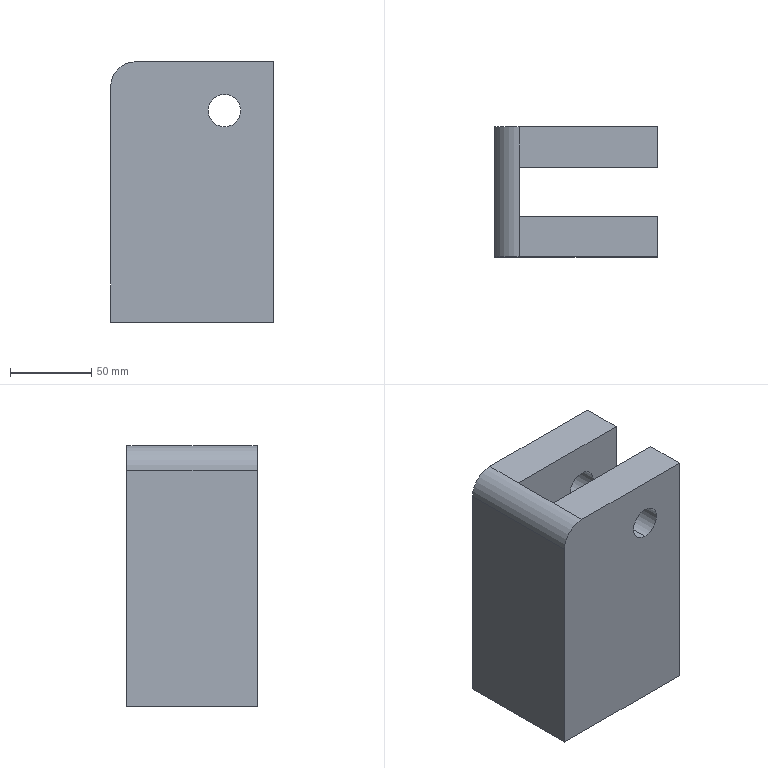Part | SolidWorks | features Cut 2, Extrusion 1, Fillet 1 | 1 solid | 16 faces | box 99.912 x 80 x 160 mm | volume 851721 mm3 | plane 11 | cylinder 5 | commonest cylinder face diameters 20 x4 30 x1
STEP:
#1=CARTESIAN_POINT('',(-55.088,-15.,140.));
#2=VERTEX_POINT('',#1);
#3=CARTESIAN_POINT('',(-55.088,-15.,120.));
#4=VERTEX_POINT('',#3);
#5=CARTESIAN_POINT('',(-55.088,-15.,130.));
#6=DIRECTION('',(0.,-1.,0.));
#7=DIRECTION('',(1.,0.,0.));
#8=AXIS2_PLACEMENT_3D('',#5,#6,#7);
#9=CIRCLE('',#8,10.);
#10=EDGE_CURVE('',#2,#4,#9,.T.);
#11=ORIENTED_EDGE('',*,*,#10,.F.);
#12=CARTESIAN_POINT('',(-55.088,-40.,140.));
#13=VERTEX_POINT('',#12);
#14=CARTESIAN_POINT('',(-55.088,120.,140.));
#15=DIRECTION('',(0.,-1.,0.));
#16=VECTOR('',#15,1000.);
#17=LINE('',#14,#16);
#18=EDGE_CURVE('',#2,#13,#17,.T.);
#19=ORIENTED_EDGE('',*,*,#18,.T.);
#20=CARTESIAN_POINT('',(-55.088,-40.,120.));
#21=VERTEX_POINT('',#20);
#22=CARTESIAN_POINT('',(-55.088,-40.,130.));
#23=DIRECTION('',(0.,-1.,0.));
#24=DIRECTION('',(0.,0.,-1.));
#25=AXIS2_PLACEMENT_3D('',#22,#23,#24);
#26=CIRCLE('',#25,10.);
#27=EDGE_CURVE('',#13,#21,#26,.T.);
#28=ORIENTED_EDGE('',*,*,#27,.T.);
#29=CARTESIAN_POINT('',(-55.088,120.,120.));
#30=DIRECTION('',(0.,-1.,0.));
#31=VECTOR('',#30,1000.);
#32=LINE('',#29,#31);
#33=EDGE_CURVE('',#4,#21,#32,.T.);
#34=ORIENTED_EDGE('',*,*,#33,.F.);
#35=EDGE_LOOP('',(#11,#19,#28,#34));
#36=FACE_OUTER_BOUND('',#35,.T.);
#37=CARTESIAN_POINT('',(-55.088,120.,130.));
#38=DIRECTION('',(0.,-1.,0.));
#39=DIRECTION('',(0.,0.,-1.));
#40=AXIS2_PLACEMENT_3D('',#37,#38,#39);
#41=CYLINDRICAL_SURFACE('',#40,10.);
#42=ADVANCED_FACE('',(#36),#41,.F.);
#43=CARTESIAN_POINT('',(-55.088,40.,140.));
#44=VERTEX_POINT('',#43);
#45=CARTESIAN_POINT('',(-55.088,40.,120.));
#46=VERTEX_POINT('',#45);
#47=CARTESIAN_POINT('',(-55.088,40.,130.));
#48=DIRECTION('',(0.,-1.,0.));
#49=DIRECTION('',(0.,0.,-1.));
#50=AXIS2_PLACEMENT_3D('',#47,#48,#49);
#51=CIRCLE('',#50,10.);
#52=EDGE_CURVE('',#44,#46,#51,.T.);
#53=ORIENTED_EDGE('',*,*,#52,.F.);
#54=CARTESIAN_POINT('',(-55.088,15.,140.));
#55=VERTEX_POINT('',#54);
#56=CARTESIAN_POINT('',(-55.088,120.,140.));
#57=DIRECTION('',(0.,-1.,0.));
#58=VECTOR('',#57,1000.);
#59=LINE('',#56,#58);
#60=EDGE_CURVE('',#44,#55,#59,.T.);
#61=ORIENTED_EDGE('',*,*,#60,.T.);
#62=CARTESIAN_POINT('',(-55.088,15.,120.));
#63=VERTEX_POINT('',#62);
#64=CARTESIAN_POINT('',(-55.088,15.,130.));
#65=DIRECTION('',(0.,1.,0.));
#66=DIRECTION('',(-1.,0.,0.));
#67=AXIS2_PLACEMENT_3D('',#64,#65,#66);
#68=CIRCLE('',#67,10.);
#69=EDGE_CURVE('',#63,#55,#68,.T.);
#70=ORIENTED_EDGE('',*,*,#69,.F.);
#71=CARTESIAN_POINT('',(-55.088,120.,120.));
#72=DIRECTION('',(0.,-1.,0.));
#73=VECTOR('',#72,1000.);
#74=LINE('',#71,#73);
#75=EDGE_CURVE('',#46,#63,#74,.T.);
#76=ORIENTED_EDGE('',*,*,#75,.F.);
#77=EDGE_LOOP('',(#53,#61,#70,#76));
#78=FACE_OUTER_BOUND('',#77,.T.);
#79=CARTESIAN_POINT('',(-55.088,120.,130.));
#80=DIRECTION('',(0.,-1.,0.));
#81=DIRECTION('',(0.,0.,-1.));
#82=AXIS2_PLACEMENT_3D('',#79,#80,#81);
#83=CYLINDRICAL_SURFACE('',#82,10.);
#84=ADVANCED_FACE('',(#78),#83,.F.);
#85=CARTESIAN_POINT('',(-25.088,40.,160.));
#86=VERTEX_POINT('',#85);
#87=CARTESIAN_POINT('',(-110.,40.,160.));
#88=VERTEX_POINT('',#87);
#89=CARTESIAN_POINT('',(-25.088,40.,160.));
#90=DIRECTION('',(-1.,0.,0.));
#91=VECTOR('',#90,1000.);
#92=LINE('',#89,#91);
#93=EDGE_CURVE('',#86,#88,#92,.T.);
#94=ORIENTED_EDGE('',*,*,#93,.T.);
#95=CARTESIAN_POINT('',(-110.,15.,160.));
#96=VERTEX_POINT('',#95);
#97=CARTESIAN_POINT('',(-110.,0.,160.));
#98=DIRECTION('',(0.,-1.,0.));
#99=VECTOR('',#98,1000.);
#100=LINE('',#97,#99);
#101=EDGE_CURVE('',#88,#96,#100,.T.);
#102=ORIENTED_EDGE('',*,*,#101,.T.);
#103=CARTESIAN_POINT('',(-25.088,15.,160.));
#104=VERTEX_POINT('',#103);
#105=CARTESIAN_POINT('',(-25.088,15.,160.));
#106=DIRECTION('',(-1.,0.,0.));
#107=VECTOR('',#106,1000.);
#108=LINE('',#105,#107);
#109=EDGE_CURVE('',#104,#96,#108,.T.);
#110=ORIENTED_EDGE('',*,*,#109,.F.);
#111=CARTESIAN_POINT('',(-25.088,40.,160.));
#112=DIRECTION('',(0.,1.,0.));
#113=VECTOR('',#112,1000.);
#114=LINE('',#111,#113);
#115=EDGE_CURVE('',#104,#86,#114,.T.);
#116=ORIENTED_EDGE('',*,*,#115,.T.);
#117=EDGE_LOOP('',(#94,#102,#110,#116));
#118=FACE_OUTER_BOUND('',#117,.T.);
#119=CARTESIAN_POINT('',(0.,0.,160.));
#120=DIRECTION('',(0.,0.,-1.));
#121=DIRECTION('',(-1.,0.,0.));
#122=AXIS2_PLACEMENT_3D('',#119,#120,#121);
#123=PLANE('',#122);
#124=ADVANCED_FACE('',(#118),#123,.F.);
#125=CARTESIAN_POINT('',(-25.088,-40.,0.));
#126=VERTEX_POINT('',#125);
#127=CARTESIAN_POINT('',(-25.088,-15.,0.));
#128=VERTEX_POINT('',#127);
#129=CARTESIAN_POINT('',(-25.088,40.,0.));
#130=DIRECTION('',(0.,1.,0.));
#131=VECTOR('',#130,1000.);
#132=LINE('',#129,#131);
#133=EDGE_CURVE('',#126,#128,#132,.T.);
#134=ORIENTED_EDGE('',*,*,#133,.T.);
#135=CARTESIAN_POINT('',(-25.088,-15.,160.));
#136=VERTEX_POINT('',#135);
#137=CARTESIAN_POINT('',(-25.088,-15.,0.));
#138=DIRECTION('',(0.,0.,1.));
#139=VECTOR('',#138,1000.);
#140=LINE('',#137,#139);
#141=EDGE_CURVE('',#128,#136,#140,.T.);
#142=ORIENTED_EDGE('',*,*,#141,.T.);
#143=CARTESIAN_POINT('',(-25.088,-40.,160.));
#144=VERTEX_POINT('',#143);
#145=CARTESIAN_POINT('',(-25.088,40.,160.));
#146=DIRECTION('',(0.,1.,0.));
#147=VECTOR('',#146,1000.);
#148=LINE('',#145,#147);
#149=EDGE_CURVE('',#144,#136,#148,.T.);
#150=ORIENTED_EDGE('',*,*,#149,.F.);
#151=CARTESIAN_POINT('',(-25.088,-40.,160.));
#152=DIRECTION('',(0.,0.,-1.));
#153=VECTOR('',#152,1000.);
#154=LINE('',#151,#153);
#155=EDGE_CURVE('',#144,#126,#154,.T.);
#156=ORIENTED_EDGE('',*,*,#155,.T.);
#157=EDGE_LOOP('',(#134,#142,#150,#156));
#158=FACE_OUTER_BOUND('',#157,.T.);
#159=CARTESIAN_POINT('',(-25.088,40.,160.));
#160=DIRECTION('',(-1.,0.,0.));
#161=DIRECTION('',(0.,-1.,0.));
#162=AXIS2_PLACEMENT_3D('',#159,#160,#161);
#163=PLANE('',#162);
#164=ADVANCED_FACE('',(#158),#163,.F.);
#165=ORIENTED_EDGE('',*,*,#115,.F.);
#166=CARTESIAN_POINT('',(-25.088,15.,0.));
#167=VERTEX_POINT('',#166);
#168=CARTESIAN_POINT('',(-25.088,15.,0.));
#169=DIRECTION('',(0.,0.,1.));
#170=VECTOR('',#169,1000.);
#171=LINE('',#168,#170);
#172=EDGE_CURVE('',#167,#104,#171,.T.);
#173=ORIENTED_EDGE('',*,*,#172,.F.);
#174=CARTESIAN_POINT('',(-25.088,40.,0.));
#175=VERTEX_POINT('',#174);
#176=CARTESIAN_POINT('',(-25.088,40.,0.));
#177=DIRECTION('',(0.,1.,0.));
#178=VECTOR('',#177,1000.);
#179=LINE('',#176,#178);
#180=EDGE_CURVE('',#167,#175,#179,.T.);
#181=ORIENTED_EDGE('',*,*,#180,.T.);
#182=CARTESIAN_POINT('',(-25.088,40.,160.));
#183=DIRECTION('',(0.,0.,-1.));
#184=VECTOR('',#183,1000.);
#185=LINE('',#182,#184);
#186=EDGE_CURVE('',#86,#175,#185,.T.);
#187=ORIENTED_EDGE('',*,*,#186,.F.);
#188=EDGE_LOOP('',(#165,#173,#181,#187));
#189=FACE_OUTER_BOUND('',#188,.T.);
#190=CARTESIAN_POINT('',(-25.088,40.,160.));
#191=DIRECTION('',(-1.,0.,0.));
#192=DIRECTION('',(0.,-1.,0.));
#193=AXIS2_PLACEMENT_3D('',#190,#191,#192);
#194=PLANE('',#193);
#195=ADVANCED_FACE('',(#189),#194,.F.);
#196=CARTESIAN_POINT('',(-55.088,40.,130.));
#197=DIRECTION('',(0.,-1.,0.));
#198=DIRECTION('',(0.,0.,-1.));
#199=AXIS2_PLACEMENT_3D('',#196,#197,#198);
#200=CIRCLE('',#199,10.);
#201=EDGE_CURVE('',#46,#44,#200,.T.);
#202=ORIENTED_EDGE('',*,*,#201,.T.);
#203=ORIENTED_EDGE('',*,*,#52,.T.);
#204=EDGE_LOOP('',(#202,#203));
#205=FACE_BOUND('',#204,.T.);
#206=CARTESIAN_POINT('',(-125.,40.,145.));
#207=VERTEX_POINT('',#206);
#208=CARTESIAN_POINT('',(-125.,40.,0.));
#209=VERTEX_POINT('',#208);
#210=CARTESIAN_POINT('',(-125.,40.,160.));
#211=DIRECTION('',(0.,0.,-1.));
#212=VECTOR('',#211,1000.);
#213=LINE('',#210,#212);
#214=EDGE_CURVE('',#207,#209,#213,.T.);
#215=ORIENTED_EDGE('',*,*,#214,.F.);
#216=CARTESIAN_POINT('',(-110.,40.,145.));
#217=DIRECTION('',(0.,1.,0.));
#218=DIRECTION('',(0.,0.,-1.));
#219=AXIS2_PLACEMENT_3D('',#216,#217,#218);
#220=CIRCLE('',#219,15.);
#221=EDGE_CURVE('',#207,#88,#220,.T.);
#222=ORIENTED_EDGE('',*,*,#221,.T.);
#223=ORIENTED_EDGE('',*,*,#93,.F.);
#224=ORIENTED_EDGE('',*,*,#186,.T.);
#225=CARTESIAN_POINT('',(-25.088,40.,0.));
#226=DIRECTION('',(-1.,0.,0.));
#227=VECTOR('',#226,1000.);
#228=LINE('',#225,#227);
#229=EDGE_CURVE('',#175,#209,#228,.T.);
#230=ORIENTED_EDGE('',*,*,#229,.T.);
#231=EDGE_LOOP('',(#215,#222,#223,#224,#230));
#232=FACE_OUTER_BOUND('',#231,.T.);
#233=CARTESIAN_POINT('',(-25.088,40.,160.));
#234=DIRECTION('',(0.,-1.,0.));
#235=DIRECTION('',(0.,0.,-1.));
#236=AXIS2_PLACEMENT_3D('',#233,#234,#235);
#237=PLANE('',#236);
#238=ADVANCED_FACE('',(#205,#232),#237,.F.);
#239=CARTESIAN_POINT('',(-125.,-40.,145.));
#240=VERTEX_POINT('',#239);
#241=CARTESIAN_POINT('',(-125.,-40.,0.));
#242=VERTEX_POINT('',#241);
#243=CARTESIAN_POINT('',(-125.,-40.,160.));
#244=DIRECTION('',(0.,0.,-1.));
#245=VECTOR('',#244,1000.);
#246=LINE('',#243,#245);
#247=EDGE_CURVE('',#240,#242,#246,.T.);
#248=ORIENTED_EDGE('',*,*,#247,.F.);
#249=CARTESIAN_POINT('',(-125.,40.,145.));
#250=DIRECTION('',(0.,1.,0.));
#251=VECTOR('',#250,1000.);
#252=LINE('',#249,#251);
#253=EDGE_CURVE('',#240,#207,#252,.T.);
#254=ORIENTED_EDGE('',*,*,#253,.T.);
#255=ORIENTED_EDGE('',*,*,#214,.T.);
#256=CARTESIAN_POINT('',(-125.,40.,0.));
#257=DIRECTION('',(0.,-1.,0.));
#258=VECTOR('',#257,1000.);
#259=LINE('',#256,#258);
#260=EDGE_CURVE('',#209,#242,#259,.T.);
#261=ORIENTED_EDGE('',*,*,#260,.T.);
#262=EDGE_LOOP('',(#248,#254,#255,#261));
#263=FACE_OUTER_BOUND('',#262,.T.);
#264=CARTESIAN_POINT('',(-125.,40.,160.));
#265=DIRECTION('',(1.,0.,0.));
#266=DIRECTION('',(0.,0.,-1.));
#267=AXIS2_PLACEMENT_3D('',#264,#265,#266);
#268=PLANE('',#267);
#269=ADVANCED_FACE('',(#263),#268,.F.);
#270=CARTESIAN_POINT('',(-55.088,-40.,130.));
#271=DIRECTION('',(0.,-1.,0.));
#272=DIRECTION('',(0.,0.,-1.));
#273=AXIS2_PLACEMENT_3D('',#270,#271,#272);
#274=CIRCLE('',#273,10.);
#275=EDGE_CURVE('',#21,#13,#274,.T.);
#276=ORIENTED_EDGE('',*,*,#275,.F.);
#277=ORIENTED_EDGE('',*,*,#27,.F.);
#278=EDGE_LOOP('',(#276,#277));
#279=FACE_BOUND('',#278,.T.);
#280=CARTESIAN_POINT('',(-110.,-40.,160.));
#281=VERTEX_POINT('',#280);
#282=CARTESIAN_POINT('',(-25.088,-40.,160.));
#283=DIRECTION('',(1.,0.,0.));
#284=VECTOR('',#283,1000.);
#285=LINE('',#282,#284);
#286=EDGE_CURVE('',#281,#144,#285,.T.);
#287=ORIENTED_EDGE('',*,*,#286,.F.);
#288=CARTESIAN_POINT('',(-110.,-40.,145.));
#289=DIRECTION('',(0.,-1.,0.));
#290=DIRECTION('',(0.,0.,1.));
#291=AXIS2_PLACEMENT_3D('',#288,#289,#290);
#292=CIRCLE('',#291,15.);
#293=EDGE_CURVE('',#281,#240,#292,.T.);
#294=ORIENTED_EDGE('',*,*,#293,.T.);
#295=ORIENTED_EDGE('',*,*,#247,.T.);
#296=CARTESIAN_POINT('',(-25.088,-40.,0.));
#297=DIRECTION('',(1.,0.,0.));
#298=VECTOR('',#297,1000.);
#299=LINE('',#296,#298);
#300=EDGE_CURVE('',#242,#126,#299,.T.);
#301=ORIENTED_EDGE('',*,*,#300,.T.);
#302=ORIENTED_EDGE('',*,*,#155,.F.);
#303=EDGE_LOOP('',(#287,#294,#295,#301,#302));
#304=FACE_OUTER_BOUND('',#303,.T.);
#305=CARTESIAN_POINT('',(-25.088,-40.,160.));
#306=DIRECTION('',(0.,1.,0.));
#307=DIRECTION('',(0.,0.,1.));
#308=AXIS2_PLACEMENT_3D('',#305,#306,#307);
#309=PLANE('',#308);
#310=ADVANCED_FACE('',(#279,#304),#309,.F.);
#311=CARTESIAN_POINT('',(-110.,-15.,160.));
#312=VERTEX_POINT('',#311);
#313=CARTESIAN_POINT('',(-110.,-15.,160.));
#314=DIRECTION('',(1.,0.,0.));
#315=VECTOR('',#314,1000.);
#316=LINE('',#313,#315);
#317=EDGE_CURVE('',#312,#136,#316,.T.);
#318=ORIENTED_EDGE('',*,*,#317,.F.);
#319=CARTESIAN_POINT('',(-110.,0.,160.));
#320=DIRECTION('',(0.,-1.,0.));
#321=VECTOR('',#320,1000.);
#322=LINE('',#319,#321);
#323=EDGE_CURVE('',#312,#281,#322,.T.);
#324=ORIENTED_EDGE('',*,*,#323,.T.);
#325=ORIENTED_EDGE('',*,*,#286,.T.);
#326=ORIENTED_EDGE('',*,*,#149,.T.);
#327=EDGE_LOOP('',(#318,#324,#325,#326));
#328=FACE_OUTER_BOUND('',#327,.T.);
#329=CARTESIAN_POINT('',(0.,0.,160.));
#330=DIRECTION('',(0.,0.,-1.));
#331=DIRECTION('',(-1.,0.,0.));
#332=AXIS2_PLACEMENT_3D('',#329,#330,#331);
#333=PLANE('',#332);
#334=ADVANCED_FACE('',(#328),#333,.F.);
#335=CARTESIAN_POINT('',(-110.,-15.,0.));
#336=VERTEX_POINT('',#335);
#337=CARTESIAN_POINT('',(-110.,-15.,0.));
#338=DIRECTION('',(1.,0.,0.));
#339=VECTOR('',#338,1000.);
#340=LINE('',#337,#339);
#341=EDGE_CURVE('',#336,#128,#340,.T.);
#342=ORIENTED_EDGE('',*,*,#341,.T.);
#343=ORIENTED_EDGE('',*,*,#133,.F.);
#344=ORIENTED_EDGE('',*,*,#300,.F.);
#345=ORIENTED_EDGE('',*,*,#260,.F.);
#346=ORIENTED_EDGE('',*,*,#229,.F.);
#347=ORIENTED_EDGE('',*,*,#180,.F.);
#348=CARTESIAN_POINT('',(-110.,15.,0.));
#349=VERTEX_POINT('',#348);
#350=CARTESIAN_POINT('',(-25.088,15.,0.));
#351=DIRECTION('',(-1.,0.,0.));
#352=VECTOR('',#351,1000.);
#353=LINE('',#350,#352);
#354=EDGE_CURVE('',#167,#349,#353,.T.);
#355=ORIENTED_EDGE('',*,*,#354,.T.);
#356=CARTESIAN_POINT('',(-110.,15.,0.));
#357=DIRECTION('',(0.,-1.,0.));
#358=VECTOR('',#357,1000.);
#359=LINE('',#356,#358);
#360=EDGE_CURVE('',#349,#336,#359,.T.);
#361=ORIENTED_EDGE('',*,*,#360,.T.);
#362=EDGE_LOOP('',(#342,#343,#344,#345,#346,#347,#355,#361));
#363=FACE_OUTER_BOUND('',#362,.T.);
#364=CARTESIAN_POINT('',(0.,0.,0.));
#365=DIRECTION('',(0.,0.,-1.));
#366=DIRECTION('',(-1.,0.,0.));
#367=AXIS2_PLACEMENT_3D('',#364,#365,#366);
#368=PLANE('',#367);
#369=ADVANCED_FACE('',(#363),#368,.T.);
#370=CARTESIAN_POINT('',(-55.088,-15.,130.));
#371=DIRECTION('',(0.,-1.,0.));
#372=DIRECTION('',(1.,0.,0.));
#373=AXIS2_PLACEMENT_3D('',#370,#371,#372);
#374=CIRCLE('',#373,10.);
#375=EDGE_CURVE('',#4,#2,#374,.T.);
#376=ORIENTED_EDGE('',*,*,#375,.T.);
#377=ORIENTED_EDGE('',*,*,#10,.T.);
#378=EDGE_LOOP('',(#376,#377));
#379=FACE_BOUND('',#378,.T.);
#380=ORIENTED_EDGE('',*,*,#317,.T.);
#381=ORIENTED_EDGE('',*,*,#141,.F.);
#382=ORIENTED_EDGE('',*,*,#341,.F.);
#383=CARTESIAN_POINT('',(-110.,-15.,0.));
#384=DIRECTION('',(0.,0.,1.));
#385=VECTOR('',#384,1000.);
#386=LINE('',#383,#385);
#387=EDGE_CURVE('',#336,#312,#386,.T.);
#388=ORIENTED_EDGE('',*,*,#387,.T.);
#389=EDGE_LOOP('',(#380,#381,#382,#388));
#390=FACE_OUTER_BOUND('',#389,.T.);
#391=CARTESIAN_POINT('',(-110.,-15.,0.));
#392=DIRECTION('',(0.,-1.,0.));
#393=DIRECTION('',(1.,0.,0.));
#394=AXIS2_PLACEMENT_3D('',#391,#392,#393);
#395=PLANE('',#394);
#396=ADVANCED_FACE('',(#379,#390),#395,.F.);
#397=CARTESIAN_POINT('',(-110.,15.,160.));
#398=DIRECTION('',(0.,-1.,0.));
#399=VECTOR('',#398,1000.);
#400=LINE('',#397,#399);
#401=EDGE_CURVE('',#96,#312,#400,.T.);
#402=ORIENTED_EDGE('',*,*,#401,.T.);
#403=ORIENTED_EDGE('',*,*,#387,.F.);
#404=ORIENTED_EDGE('',*,*,#360,.F.);
#405=CARTESIAN_POINT('',(-110.,15.,0.));
#406=DIRECTION('',(0.,0.,1.));
#407=VECTOR('',#406,1000.);
#408=LINE('',#405,#407);
#409=EDGE_CURVE('',#349,#96,#408,.T.);
#410=ORIENTED_EDGE('',*,*,#409,.T.);
#411=EDGE_LOOP('',(#402,#403,#404,#410));
#412=FACE_OUTER_BOUND('',#411,.T.);
#413=CARTESIAN_POINT('',(-110.,15.,0.));
#414=DIRECTION('',(-1.,0.,0.));
#415=DIRECTION('',(0.,0.,1.));
#416=AXIS2_PLACEMENT_3D('',#413,#414,#415);
#417=PLANE('',#416);
#418=ADVANCED_FACE('',(#412),#417,.F.);
#419=ORIENTED_EDGE('',*,*,#69,.T.);
#420=CARTESIAN_POINT('',(-55.088,15.,130.));
#421=DIRECTION('',(0.,1.,0.));
#422=DIRECTION('',(-1.,0.,0.));
#423=AXIS2_PLACEMENT_3D('',#420,#421,#422);
#424=CIRCLE('',#423,10.);
#425=EDGE_CURVE('',#55,#63,#424,.T.);
#426=ORIENTED_EDGE('',*,*,#425,.T.);
#427=EDGE_LOOP('',(#419,#426));
#428=FACE_BOUND('',#427,.T.);
#429=ORIENTED_EDGE('',*,*,#109,.T.);
#430=ORIENTED_EDGE('',*,*,#409,.F.);
#431=ORIENTED_EDGE('',*,*,#354,.F.);
#432=ORIENTED_EDGE('',*,*,#172,.T.);
#433=EDGE_LOOP('',(#429,#430,#431,#432));
#434=FACE_OUTER_BOUND('',#433,.T.);
#435=CARTESIAN_POINT('',(-25.088,15.,0.));
#436=DIRECTION('',(0.,1.,0.));
#437=DIRECTION('',(-1.,0.,0.));
#438=AXIS2_PLACEMENT_3D('',#435,#436,#437);
#439=PLANE('',#438);
#440=ADVANCED_FACE('',(#428,#434),#439,.F.);
#441=ORIENTED_EDGE('',*,*,#221,.F.);
#442=ORIENTED_EDGE('',*,*,#253,.F.);
#443=ORIENTED_EDGE('',*,*,#293,.F.);
#444=ORIENTED_EDGE('',*,*,#323,.F.);
#445=ORIENTED_EDGE('',*,*,#401,.F.);
#446=ORIENTED_EDGE('',*,*,#101,.F.);
#447=EDGE_LOOP('',(#441,#442,#443,#444,#445,#446));
#448=FACE_OUTER_BOUND('',#447,.T.);
#449=CARTESIAN_POINT('',(-110.,0.,145.));
#450=DIRECTION('',(0.,-1.,0.));
#451=DIRECTION('',(0.,0.,-1.));
#452=AXIS2_PLACEMENT_3D('',#449,#450,#451);
#453=CYLINDRICAL_SURFACE('',#452,15.);
#454=ADVANCED_FACE('',(#448),#453,.T.);
#455=ORIENTED_EDGE('',*,*,#60,.F.);
#456=ORIENTED_EDGE('',*,*,#201,.F.);
#457=ORIENTED_EDGE('',*,*,#75,.T.);
#458=ORIENTED_EDGE('',*,*,#425,.F.);
#459=EDGE_LOOP('',(#455,#456,#457,#458));
#460=FACE_OUTER_BOUND('',#459,.T.);
#461=CARTESIAN_POINT('',(-55.088,120.,130.));
#462=DIRECTION('',(0.,-1.,0.));
#463=DIRECTION('',(0.,0.,-1.));
#464=AXIS2_PLACEMENT_3D('',#461,#462,#463);
#465=CYLINDRICAL_SURFACE('',#464,10.);
#466=ADVANCED_FACE('',(#460),#465,.F.);
#467=ORIENTED_EDGE('',*,*,#18,.F.);
#468=ORIENTED_EDGE('',*,*,#375,.F.);
#469=ORIENTED_EDGE('',*,*,#33,.T.);
#470=ORIENTED_EDGE('',*,*,#275,.T.);
#471=EDGE_LOOP('',(#467,#468,#469,#470));
#472=FACE_OUTER_BOUND('',#471,.T.);
#473=CARTESIAN_POINT('',(-55.088,120.,130.));
#474=DIRECTION('',(0.,-1.,0.));
#475=DIRECTION('',(0.,0.,-1.));
#476=AXIS2_PLACEMENT_3D('',#473,#474,#475);
#477=CYLINDRICAL_SURFACE('',#476,10.);
#478=ADVANCED_FACE('',(#472),#477,.F.);
#479=CLOSED_SHELL('',(#42,#84,#124,#164,#195,#238,#269,#310,#334,#369,#396,#418,#440,#454,#466,#478));
#480=MANIFOLD_SOLID_BREP('',#479);
#481=CARTESIAN_POINT('',(0.,0.,0.));
#482=DIRECTION('',(0.,0.,1.));
#483=DIRECTION('',(1.,0.,0.));
#484=AXIS2_PLACEMENT_3D('',#481,#482,#483);
#485=(LENGTH_UNIT()NAMED_UNIT(*)SI_UNIT(.MILLI.,.METRE.));
#486=UNCERTAINTY_MEASURE_WITH_UNIT(LENGTH_MEASURE(0.00001),#485,'','');
#487=(NAMED_UNIT(*)PLANE_ANGLE_UNIT()SI_UNIT($,.RADIAN.));
#488=(NAMED_UNIT(*)SI_UNIT($,.STERADIAN.)SOLID_ANGLE_UNIT());
#489=(GEOMETRIC_REPRESENTATION_CONTEXT(3)GLOBAL_UNCERTAINTY_ASSIGNED_CONTEXT((#486))GLOBAL_UNIT_ASSIGNED_CONTEXT((#485,#487,#488))REPRESENTATION_CONTEXT('',''));
#490=ADVANCED_BREP_SHAPE_REPRESENTATION('',(#480,#484),#489);